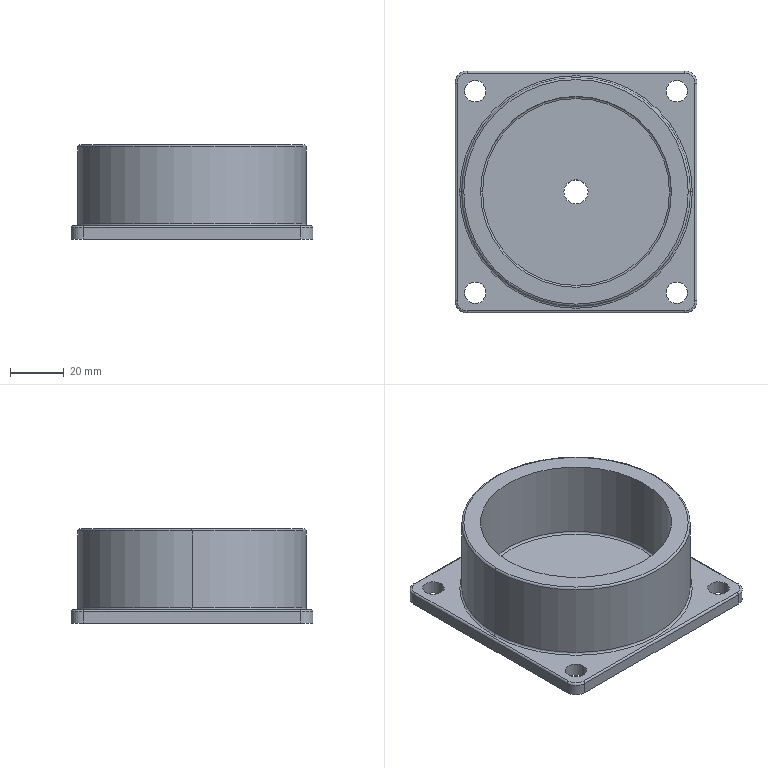Part | SolidWorks | features ICE 4, Extrusion 1, Fillet 1, Scale 1 | 1 solid | 40 faces | box 90 x 90 x 35 mm | volume 90534 mm3 | cylinder 22 | torus 10 | plane 8 | commonest cylinder face diameters 8 x8 9 x6 1.5 x4 71 x2 85 x2
STEP:
#1=CARTESIAN_POINT('',(1.319,-1.476,0.1969));
#2=VERTEX_POINT('',#1);
#3=CARTESIAN_POINT('',(1.634,-1.476,0.1969));
#4=VERTEX_POINT('',#3);
#5=CARTESIAN_POINT('',(1.476,-1.476,0.1969));
#6=DIRECTION('',(0.,0.,1.));
#7=DIRECTION('',(1.,0.,0.));
#8=AXIS2_PLACEMENT_3D('',#5,#6,#7);
#9=CIRCLE('',#8,0.1575);
#10=EDGE_CURVE('',#2,#4,#9,.T.);
#11=ORIENTED_EDGE('',*,*,#10,.T.);
#12=CARTESIAN_POINT('',(1.634,-1.476,0.));
#13=VERTEX_POINT('',#12);
#14=CARTESIAN_POINT('',(1.634,-1.476,0.3937));
#15=DIRECTION('',(0.,0.,-1.));
#16=VECTOR('',#15,39.37);
#17=LINE('',#14,#16);
#18=EDGE_CURVE('',#4,#13,#17,.T.);
#19=ORIENTED_EDGE('',*,*,#18,.T.);
#20=CARTESIAN_POINT('',(1.319,-1.476,0.));
#21=VERTEX_POINT('',#20);
#22=CARTESIAN_POINT('',(1.476,-1.476,0.));
#23=DIRECTION('',(0.,0.,-1.));
#24=DIRECTION('',(1.,0.,0.));
#25=AXIS2_PLACEMENT_3D('',#22,#23,#24);
#26=CIRCLE('',#25,0.1575);
#27=EDGE_CURVE('',#13,#21,#26,.T.);
#28=ORIENTED_EDGE('',*,*,#27,.T.);
#29=CARTESIAN_POINT('',(1.319,-1.476,0.3937));
#30=DIRECTION('',(0.,0.,-1.));
#31=VECTOR('',#30,39.37);
#32=LINE('',#29,#31);
#33=EDGE_CURVE('',#2,#21,#32,.T.);
#34=ORIENTED_EDGE('',*,*,#33,.F.);
#35=EDGE_LOOP('',(#11,#19,#28,#34));
#36=FACE_OUTER_BOUND('',#35,.T.);
#37=CARTESIAN_POINT('',(1.476,-1.476,0.3937));
#38=DIRECTION('',(0.,0.,-1.));
#39=DIRECTION('',(-1.,0.,0.));
#40=AXIS2_PLACEMENT_3D('',#37,#38,#39);
#41=CYLINDRICAL_SURFACE('',#40,0.1575);
#42=ADVANCED_FACE('',(#36),#41,.F.);
#43=CARTESIAN_POINT('',(-1.634,1.476,0.1969));
#44=VERTEX_POINT('',#43);
#45=CARTESIAN_POINT('',(-1.319,1.476,0.1969));
#46=VERTEX_POINT('',#45);
#47=CARTESIAN_POINT('',(-1.476,1.476,0.1969));
#48=DIRECTION('',(0.,0.,1.));
#49=DIRECTION('',(1.,0.,0.));
#50=AXIS2_PLACEMENT_3D('',#47,#48,#49);
#51=CIRCLE('',#50,0.1575);
#52=EDGE_CURVE('',#44,#46,#51,.T.);
#53=ORIENTED_EDGE('',*,*,#52,.T.);
#54=CARTESIAN_POINT('',(-1.319,1.476,0.));
#55=VERTEX_POINT('',#54);
#56=CARTESIAN_POINT('',(-1.319,1.476,0.3937));
#57=DIRECTION('',(0.,0.,-1.));
#58=VECTOR('',#57,39.37);
#59=LINE('',#56,#58);
#60=EDGE_CURVE('',#46,#55,#59,.T.);
#61=ORIENTED_EDGE('',*,*,#60,.T.);
#62=CARTESIAN_POINT('',(-1.634,1.476,0.));
#63=VERTEX_POINT('',#62);
#64=CARTESIAN_POINT('',(-1.476,1.476,0.));
#65=DIRECTION('',(0.,0.,-1.));
#66=DIRECTION('',(1.,0.,0.));
#67=AXIS2_PLACEMENT_3D('',#64,#65,#66);
#68=CIRCLE('',#67,0.1575);
#69=EDGE_CURVE('',#55,#63,#68,.T.);
#70=ORIENTED_EDGE('',*,*,#69,.T.);
#71=CARTESIAN_POINT('',(-1.634,1.476,0.3937));
#72=DIRECTION('',(0.,0.,-1.));
#73=VECTOR('',#72,39.37);
#74=LINE('',#71,#73);
#75=EDGE_CURVE('',#44,#63,#74,.T.);
#76=ORIENTED_EDGE('',*,*,#75,.F.);
#77=EDGE_LOOP('',(#53,#61,#70,#76));
#78=FACE_OUTER_BOUND('',#77,.T.);
#79=CARTESIAN_POINT('',(-1.476,1.476,0.3937));
#80=DIRECTION('',(0.,0.,-1.));
#81=DIRECTION('',(-1.,0.,0.));
#82=AXIS2_PLACEMENT_3D('',#79,#80,#81);
#83=CYLINDRICAL_SURFACE('',#82,0.1575);
#84=ADVANCED_FACE('',(#78),#83,.F.);
#85=CARTESIAN_POINT('',(-1.634,-1.476,0.1969));
#86=VERTEX_POINT('',#85);
#87=CARTESIAN_POINT('',(-1.319,-1.476,0.1969));
#88=VERTEX_POINT('',#87);
#89=CARTESIAN_POINT('',(-1.476,-1.476,0.1969));
#90=DIRECTION('',(0.,0.,1.));
#91=DIRECTION('',(1.,0.,0.));
#92=AXIS2_PLACEMENT_3D('',#89,#90,#91);
#93=CIRCLE('',#92,0.1575);
#94=EDGE_CURVE('',#86,#88,#93,.T.);
#95=ORIENTED_EDGE('',*,*,#94,.T.);
#96=CARTESIAN_POINT('',(-1.319,-1.476,0.));
#97=VERTEX_POINT('',#96);
#98=CARTESIAN_POINT('',(-1.319,-1.476,0.3937));
#99=DIRECTION('',(0.,0.,-1.));
#100=VECTOR('',#99,39.37);
#101=LINE('',#98,#100);
#102=EDGE_CURVE('',#88,#97,#101,.T.);
#103=ORIENTED_EDGE('',*,*,#102,.T.);
#104=CARTESIAN_POINT('',(-1.634,-1.476,0.));
#105=VERTEX_POINT('',#104);
#106=CARTESIAN_POINT('',(-1.476,-1.476,0.));
#107=DIRECTION('',(0.,0.,-1.));
#108=DIRECTION('',(-1.,0.,0.));
#109=AXIS2_PLACEMENT_3D('',#106,#107,#108);
#110=CIRCLE('',#109,0.1575);
#111=EDGE_CURVE('',#97,#105,#110,.T.);
#112=ORIENTED_EDGE('',*,*,#111,.T.);
#113=CARTESIAN_POINT('',(-1.634,-1.476,0.3937));
#114=DIRECTION('',(0.,0.,-1.));
#115=VECTOR('',#114,39.37);
#116=LINE('',#113,#115);
#117=EDGE_CURVE('',#86,#105,#116,.T.);
#118=ORIENTED_EDGE('',*,*,#117,.F.);
#119=EDGE_LOOP('',(#95,#103,#112,#118));
#120=FACE_OUTER_BOUND('',#119,.T.);
#121=CARTESIAN_POINT('',(-1.476,-1.476,0.3937));
#122=DIRECTION('',(0.,0.,-1.));
#123=DIRECTION('',(-1.,0.,0.));
#124=AXIS2_PLACEMENT_3D('',#121,#122,#123);
#125=CYLINDRICAL_SURFACE('',#124,0.1575);
#126=ADVANCED_FACE('',(#120),#125,.F.);
#127=CARTESIAN_POINT('',(1.319,1.476,0.1969));
#128=VERTEX_POINT('',#127);
#129=CARTESIAN_POINT('',(1.634,1.476,0.1969));
#130=VERTEX_POINT('',#129);
#131=CARTESIAN_POINT('',(1.476,1.476,0.1969));
#132=DIRECTION('',(0.,0.,1.));
#133=DIRECTION('',(1.,0.,0.));
#134=AXIS2_PLACEMENT_3D('',#131,#132,#133);
#135=CIRCLE('',#134,0.1575);
#136=EDGE_CURVE('',#128,#130,#135,.T.);
#137=ORIENTED_EDGE('',*,*,#136,.T.);
#138=CARTESIAN_POINT('',(1.634,1.476,0.));
#139=VERTEX_POINT('',#138);
#140=CARTESIAN_POINT('',(1.634,1.476,0.3937));
#141=DIRECTION('',(0.,0.,-1.));
#142=VECTOR('',#141,39.37);
#143=LINE('',#140,#142);
#144=EDGE_CURVE('',#130,#139,#143,.T.);
#145=ORIENTED_EDGE('',*,*,#144,.T.);
#146=CARTESIAN_POINT('',(1.319,1.476,0.));
#147=VERTEX_POINT('',#146);
#148=CARTESIAN_POINT('',(1.476,1.476,0.));
#149=DIRECTION('',(0.,0.,-1.));
#150=DIRECTION('',(-1.,0.,0.));
#151=AXIS2_PLACEMENT_3D('',#148,#149,#150);
#152=CIRCLE('',#151,0.1575);
#153=EDGE_CURVE('',#139,#147,#152,.T.);
#154=ORIENTED_EDGE('',*,*,#153,.T.);
#155=CARTESIAN_POINT('',(1.319,1.476,0.3937));
#156=DIRECTION('',(0.,0.,-1.));
#157=VECTOR('',#156,39.37);
#158=LINE('',#155,#157);
#159=EDGE_CURVE('',#128,#147,#158,.T.);
#160=ORIENTED_EDGE('',*,*,#159,.F.);
#161=EDGE_LOOP('',(#137,#145,#154,#160));
#162=FACE_OUTER_BOUND('',#161,.T.);
#163=CARTESIAN_POINT('',(1.476,1.476,0.3937));
#164=DIRECTION('',(0.,0.,-1.));
#165=DIRECTION('',(-1.,0.,0.));
#166=AXIS2_PLACEMENT_3D('',#163,#164,#165);
#167=CYLINDRICAL_SURFACE('',#166,0.1575);
#168=ADVANCED_FACE('',(#162),#167,.F.);
#169=CARTESIAN_POINT('',(-1.673,0.,0.2264));
#170=VERTEX_POINT('',#169);
#171=CARTESIAN_POINT('',(1.673,0.,0.2264));
#172=VERTEX_POINT('',#171);
#173=CARTESIAN_POINT('',(0.,0.,0.2264));
#174=DIRECTION('',(0.,0.,1.));
#175=DIRECTION('',(1.,0.,0.));
#176=AXIS2_PLACEMENT_3D('',#173,#174,#175);
#177=CIRCLE('',#176,1.673);
#178=EDGE_CURVE('',#170,#172,#177,.T.);
#179=ORIENTED_EDGE('',*,*,#178,.F.);
#180=CARTESIAN_POINT('',(-1.703,0.,0.1969));
#181=VERTEX_POINT('',#180);
#182=CARTESIAN_POINT('',(-1.703,0.,0.2264));
#183=DIRECTION('',(0.,1.,0.));
#184=DIRECTION('',(-1.,0.,0.));
#185=AXIS2_PLACEMENT_3D('',#182,#183,#184);
#186=CIRCLE('',#185,0.02953);
#187=EDGE_CURVE('',#170,#181,#186,.T.);
#188=ORIENTED_EDGE('',*,*,#187,.T.);
#189=CARTESIAN_POINT('',(1.703,0.,0.1969));
#190=VERTEX_POINT('',#189);
#191=CARTESIAN_POINT('',(0.,0.,0.1969));
#192=DIRECTION('',(0.,0.,-1.));
#193=DIRECTION('',(1.,0.,0.));
#194=AXIS2_PLACEMENT_3D('',#191,#192,#193);
#195=CIRCLE('',#194,1.703);
#196=EDGE_CURVE('',#190,#181,#195,.T.);
#197=ORIENTED_EDGE('',*,*,#196,.F.);
#198=CARTESIAN_POINT('',(1.703,0.,0.2264));
#199=DIRECTION('',(0.,-1.,0.));
#200=DIRECTION('',(0.,0.,-1.));
#201=AXIS2_PLACEMENT_3D('',#198,#199,#200);
#202=CIRCLE('',#201,0.02953);
#203=EDGE_CURVE('',#172,#190,#202,.T.);
#204=ORIENTED_EDGE('',*,*,#203,.F.);
#205=EDGE_LOOP('',(#179,#188,#197,#204));
#206=FACE_OUTER_BOUND('',#205,.T.);
#207=CARTESIAN_POINT('',(0.,0.,0.2264));
#208=DIRECTION('',(0.,0.,1.));
#209=DIRECTION('',(1.,0.,0.));
#210=AXIS2_PLACEMENT_3D('',#207,#208,#209);
#211=TOROIDAL_SURFACE('',#210,1.703,0.02953);
#212=ADVANCED_FACE('',(#206),#211,.F.);
#213=CARTESIAN_POINT('',(-1.368,0.,0.1969));
#214=VERTEX_POINT('',#213);
#215=CARTESIAN_POINT('',(1.368,0.,0.1969));
#216=VERTEX_POINT('',#215);
#217=CARTESIAN_POINT('',(0.,0.,0.1969));
#218=DIRECTION('',(0.,0.,1.));
#219=DIRECTION('',(1.,0.,0.));
#220=AXIS2_PLACEMENT_3D('',#217,#218,#219);
#221=CIRCLE('',#220,1.368);
#222=EDGE_CURVE('',#214,#216,#221,.T.);
#223=ORIENTED_EDGE('',*,*,#222,.F.);
#224=CARTESIAN_POINT('',(-1.398,0.,0.2264));
#225=VERTEX_POINT('',#224);
#226=CARTESIAN_POINT('',(-1.368,0.,0.2264));
#227=DIRECTION('',(0.,1.,0.));
#228=DIRECTION('',(-1.,0.,0.));
#229=AXIS2_PLACEMENT_3D('',#226,#227,#228);
#230=CIRCLE('',#229,0.02953);
#231=EDGE_CURVE('',#214,#225,#230,.T.);
#232=ORIENTED_EDGE('',*,*,#231,.T.);
#233=CARTESIAN_POINT('',(1.398,0.,0.2264));
#234=VERTEX_POINT('',#233);
#235=CARTESIAN_POINT('',(0.,0.,0.2264));
#236=DIRECTION('',(0.,0.,-1.));
#237=DIRECTION('',(1.,0.,0.));
#238=AXIS2_PLACEMENT_3D('',#235,#236,#237);
#239=CIRCLE('',#238,1.398);
#240=EDGE_CURVE('',#234,#225,#239,.T.);
#241=ORIENTED_EDGE('',*,*,#240,.F.);
#242=CARTESIAN_POINT('',(1.368,0.,0.2264));
#243=DIRECTION('',(0.,-1.,0.));
#244=DIRECTION('',(0.,0.,-1.));
#245=AXIS2_PLACEMENT_3D('',#242,#243,#244);
#246=CIRCLE('',#245,0.02953);
#247=EDGE_CURVE('',#216,#234,#246,.T.);
#248=ORIENTED_EDGE('',*,*,#247,.F.);
#249=EDGE_LOOP('',(#223,#232,#241,#248));
#250=FACE_OUTER_BOUND('',#249,.T.);
#251=CARTESIAN_POINT('',(0.,0.,0.2264));
#252=DIRECTION('',(0.,0.,1.));
#253=DIRECTION('',(1.,0.,0.));
#254=AXIS2_PLACEMENT_3D('',#251,#252,#253);
#255=TOROIDAL_SURFACE('',#254,1.368,0.02953);
#256=ADVANCED_FACE('',(#250),#255,.F.);
#257=CARTESIAN_POINT('',(-1.673,0.,1.348));
#258=VERTEX_POINT('',#257);
#259=CARTESIAN_POINT('',(1.673,0.,1.348));
#260=VERTEX_POINT('',#259);
#261=CARTESIAN_POINT('',(0.,0.,1.348));
#262=DIRECTION('',(0.,0.,-1.));
#263=DIRECTION('',(1.,0.,0.));
#264=AXIS2_PLACEMENT_3D('',#261,#262,#263);
#265=CIRCLE('',#264,1.673);
#266=EDGE_CURVE('',#258,#260,#265,.T.);
#267=ORIENTED_EDGE('',*,*,#266,.F.);
#268=CARTESIAN_POINT('',(-1.644,0.,1.378));
#269=VERTEX_POINT('',#268);
#270=CARTESIAN_POINT('',(-1.644,0.,1.348));
#271=DIRECTION('',(0.,1.,0.));
#272=DIRECTION('',(-1.,0.,0.));
#273=AXIS2_PLACEMENT_3D('',#270,#271,#272);
#274=CIRCLE('',#273,0.02953);
#275=EDGE_CURVE('',#258,#269,#274,.T.);
#276=ORIENTED_EDGE('',*,*,#275,.T.);
#277=CARTESIAN_POINT('',(1.644,0.,1.378));
#278=VERTEX_POINT('',#277);
#279=CARTESIAN_POINT('',(0.,0.,1.378));
#280=DIRECTION('',(0.,0.,1.));
#281=DIRECTION('',(1.,0.,0.));
#282=AXIS2_PLACEMENT_3D('',#279,#280,#281);
#283=CIRCLE('',#282,1.644);
#284=EDGE_CURVE('',#278,#269,#283,.T.);
#285=ORIENTED_EDGE('',*,*,#284,.F.);
#286=CARTESIAN_POINT('',(1.644,0.,1.348));
#287=DIRECTION('',(0.,-1.,0.));
#288=DIRECTION('',(0.,0.,-1.));
#289=AXIS2_PLACEMENT_3D('',#286,#287,#288);
#290=CIRCLE('',#289,0.02953);
#291=EDGE_CURVE('',#260,#278,#290,.T.);
#292=ORIENTED_EDGE('',*,*,#291,.F.);
#293=EDGE_LOOP('',(#267,#276,#285,#292));
#294=FACE_OUTER_BOUND('',#293,.T.);
#295=CARTESIAN_POINT('',(0.,0.,1.348));
#296=DIRECTION('',(0.,0.,1.));
#297=DIRECTION('',(1.,0.,0.));
#298=AXIS2_PLACEMENT_3D('',#295,#296,#297);
#299=TOROIDAL_SURFACE('',#298,1.644,0.02953);
#300=ADVANCED_FACE('',(#294),#299,.T.);
#301=ORIENTED_EDGE('',*,*,#240,.T.);
#302=CARTESIAN_POINT('',(-1.398,0.,1.378));
#303=VERTEX_POINT('',#302);
#304=CARTESIAN_POINT('',(-1.398,0.,0.1969));
#305=DIRECTION('',(0.,0.,1.));
#306=VECTOR('',#305,39.37);
#307=LINE('',#304,#306);
#308=EDGE_CURVE('',#225,#303,#307,.T.);
#309=ORIENTED_EDGE('',*,*,#308,.T.);
#310=CARTESIAN_POINT('',(1.398,0.,1.378));
#311=VERTEX_POINT('',#310);
#312=CARTESIAN_POINT('',(0.,0.,1.378));
#313=DIRECTION('',(0.,0.,1.));
#314=DIRECTION('',(1.,0.,0.));
#315=AXIS2_PLACEMENT_3D('',#312,#313,#314);
#316=CIRCLE('',#315,1.398);
#317=EDGE_CURVE('',#303,#311,#316,.T.);
#318=ORIENTED_EDGE('',*,*,#317,.T.);
#319=CARTESIAN_POINT('',(1.398,0.,0.1969));
#320=DIRECTION('',(0.,0.,1.));
#321=VECTOR('',#320,39.37);
#322=LINE('',#319,#321);
#323=EDGE_CURVE('',#234,#311,#322,.T.);
#324=ORIENTED_EDGE('',*,*,#323,.F.);
#325=EDGE_LOOP('',(#301,#309,#318,#324));
#326=FACE_OUTER_BOUND('',#325,.T.);
#327=CARTESIAN_POINT('',(0.,0.,0.1969));
#328=DIRECTION('',(0.,0.,1.));
#329=DIRECTION('',(1.,0.,0.));
#330=AXIS2_PLACEMENT_3D('',#327,#328,#329);
#331=CYLINDRICAL_SURFACE('',#330,1.398);
#332=ADVANCED_FACE('',(#326),#331,.F.);
#333=ORIENTED_EDGE('',*,*,#266,.T.);
#334=CARTESIAN_POINT('',(1.673,0.,1.378));
#335=DIRECTION('',(0.,0.,-1.));
#336=VECTOR('',#335,39.37);
#337=LINE('',#334,#336);
#338=EDGE_CURVE('',#260,#172,#337,.T.);
#339=ORIENTED_EDGE('',*,*,#338,.T.);
#340=CARTESIAN_POINT('',(0.,0.,0.2264));
#341=DIRECTION('',(0.,0.,1.));
#342=DIRECTION('',(1.,0.,0.));
#343=AXIS2_PLACEMENT_3D('',#340,#341,#342);
#344=CIRCLE('',#343,1.673);
#345=EDGE_CURVE('',#172,#170,#344,.T.);
#346=ORIENTED_EDGE('',*,*,#345,.T.);
#347=CARTESIAN_POINT('',(-1.673,0.,1.378));
#348=DIRECTION('',(0.,0.,-1.));
#349=VECTOR('',#348,39.37);
#350=LINE('',#347,#349);
#351=EDGE_CURVE('',#258,#170,#350,.T.);
#352=ORIENTED_EDGE('',*,*,#351,.F.);
#353=EDGE_LOOP('',(#333,#339,#346,#352));
#354=FACE_OUTER_BOUND('',#353,.T.);
#355=CARTESIAN_POINT('',(0.,0.,1.378));
#356=DIRECTION('',(0.,0.,-1.));
#357=DIRECTION('',(-1.,0.,0.));
#358=AXIS2_PLACEMENT_3D('',#355,#356,#357);
#359=CYLINDRICAL_SURFACE('',#358,1.673);
#360=ADVANCED_FACE('',(#354),#359,.T.);
#361=CARTESIAN_POINT('',(-0.1772,0.,0.1969));
#362=VERTEX_POINT('',#361);
#363=CARTESIAN_POINT('',(0.1772,0.,0.1969));
#364=VERTEX_POINT('',#363);
#365=CARTESIAN_POINT('',(0.,0.,0.1969));
#366=DIRECTION('',(0.,0.,1.));
#367=DIRECTION('',(1.,0.,0.));
#368=AXIS2_PLACEMENT_3D('',#365,#366,#367);
#369=CIRCLE('',#368,0.1772);
#370=EDGE_CURVE('',#362,#364,#369,.T.);
#371=ORIENTED_EDGE('',*,*,#370,.T.);
#372=CARTESIAN_POINT('',(0.1772,0.,0.));
#373=VERTEX_POINT('',#372);
#374=CARTESIAN_POINT('',(0.1772,0.,0.1969));
#375=DIRECTION('',(0.,0.,-1.));
#376=VECTOR('',#375,39.37);
#377=LINE('',#374,#376);
#378=EDGE_CURVE('',#364,#373,#377,.T.);
#379=ORIENTED_EDGE('',*,*,#378,.T.);
#380=CARTESIAN_POINT('',(-0.1772,0.,0.));
#381=VERTEX_POINT('',#380);
#382=CARTESIAN_POINT('',(0.,0.,0.));
#383=DIRECTION('',(0.,0.,1.));
#384=DIRECTION('',(1.,0.,0.));
#385=AXIS2_PLACEMENT_3D('',#382,#383,#384);
#386=CIRCLE('',#385,0.1772);
#387=EDGE_CURVE('',#381,#373,#386,.T.);
#388=ORIENTED_EDGE('',*,*,#387,.F.);
#389=CARTESIAN_POINT('',(-0.1772,0.,0.1969));
#390=DIRECTION('',(0.,0.,-1.));
#391=VECTOR('',#390,39.37);
#392=LINE('',#389,#391);
#393=EDGE_CURVE('',#362,#381,#392,.T.);
#394=ORIENTED_EDGE('',*,*,#393,.F.);
#395=EDGE_LOOP('',(#371,#379,#388,#394));
#396=FACE_OUTER_BOUND('',#395,.T.);
#397=CARTESIAN_POINT('',(0.,0.,0.1969));
#398=DIRECTION('',(0.,0.,-1.));
#399=DIRECTION('',(-1.,0.,0.));
#400=AXIS2_PLACEMENT_3D('',#397,#398,#399);
#401=CYLINDRICAL_SURFACE('',#400,0.1772);
#402=ADVANCED_FACE('',(#396),#401,.F.);
#403=ORIENTED_EDGE('',*,*,#10,.F.);
#404=CARTESIAN_POINT('',(1.476,-1.476,0.1969));
#405=DIRECTION('',(0.,0.,1.));
#406=DIRECTION('',(1.,0.,0.));
#407=AXIS2_PLACEMENT_3D('',#404,#405,#406);
#408=CIRCLE('',#407,0.1575);
#409=EDGE_CURVE('',#4,#2,#408,.T.);
#410=ORIENTED_EDGE('',*,*,#409,.F.);
#411=EDGE_LOOP('',(#403,#410));
#412=FACE_BOUND('',#411,.T.);
#413=ORIENTED_EDGE('',*,*,#52,.F.);
#414=CARTESIAN_POINT('',(-1.476,1.476,0.1969));
#415=DIRECTION('',(0.,0.,1.));
#416=DIRECTION('',(1.,0.,0.));
#417=AXIS2_PLACEMENT_3D('',#414,#415,#416);
#418=CIRCLE('',#417,0.1575);
#419=EDGE_CURVE('',#46,#44,#418,.T.);
#420=ORIENTED_EDGE('',*,*,#419,.F.);
#421=EDGE_LOOP('',(#413,#420));
#422=FACE_BOUND('',#421,.T.);
#423=ORIENTED_EDGE('',*,*,#94,.F.);
#424=CARTESIAN_POINT('',(-1.476,-1.476,0.1969));
#425=DIRECTION('',(0.,0.,1.));
#426=DIRECTION('',(1.,0.,0.));
#427=AXIS2_PLACEMENT_3D('',#424,#425,#426);
#428=CIRCLE('',#427,0.1575);
#429=EDGE_CURVE('',#88,#86,#428,.T.);
#430=ORIENTED_EDGE('',*,*,#429,.F.);
#431=EDGE_LOOP('',(#423,#430));
#432=FACE_BOUND('',#431,.T.);
#433=ORIENTED_EDGE('',*,*,#136,.F.);
#434=CARTESIAN_POINT('',(1.476,1.476,0.1969));
#435=DIRECTION('',(0.,0.,1.));
#436=DIRECTION('',(1.,0.,0.));
#437=AXIS2_PLACEMENT_3D('',#434,#435,#436);
#438=CIRCLE('',#437,0.1575);
#439=EDGE_CURVE('',#130,#128,#438,.T.);
#440=ORIENTED_EDGE('',*,*,#439,.F.);
#441=EDGE_LOOP('',(#433,#440));
#442=FACE_BOUND('',#441,.T.);
#443=CARTESIAN_POINT('',(-1.594,-1.742,0.1969));
#444=VERTEX_POINT('',#443);
#445=CARTESIAN_POINT('',(1.594,-1.742,0.1969));
#446=VERTEX_POINT('',#445);
#447=CARTESIAN_POINT('',(1.594,-1.742,0.1969));
#448=DIRECTION('',(1.,0.,0.));
#449=VECTOR('',#448,39.37);
#450=LINE('',#447,#449);
#451=EDGE_CURVE('',#444,#446,#450,.T.);
#452=ORIENTED_EDGE('',*,*,#451,.T.);
#453=CARTESIAN_POINT('',(1.742,-1.594,0.1969));
#454=VERTEX_POINT('',#453);
#455=CARTESIAN_POINT('',(1.594,-1.594,0.1969));
#456=DIRECTION('',(0.,0.,1.));
#457=DIRECTION('',(1.,0.,0.));
#458=AXIS2_PLACEMENT_3D('',#455,#456,#457);
#459=CIRCLE('',#458,0.1476);
#460=EDGE_CURVE('',#446,#454,#459,.T.);
#461=ORIENTED_EDGE('',*,*,#460,.T.);
#462=CARTESIAN_POINT('',(1.742,1.594,0.1969));
#463=VERTEX_POINT('',#462);
#464=CARTESIAN_POINT('',(1.742,1.594,0.1969));
#465=DIRECTION('',(0.,1.,0.));
#466=VECTOR('',#465,39.37);
#467=LINE('',#464,#466);
#468=EDGE_CURVE('',#454,#463,#467,.T.);
#469=ORIENTED_EDGE('',*,*,#468,.T.);
#470=CARTESIAN_POINT('',(1.594,1.742,0.1969));
#471=VERTEX_POINT('',#470);
#472=CARTESIAN_POINT('',(1.594,1.594,0.1969));
#473=DIRECTION('',(0.,0.,1.));
#474=DIRECTION('',(1.,0.,0.));
#475=AXIS2_PLACEMENT_3D('',#472,#473,#474);
#476=CIRCLE('',#475,0.1476);
#477=EDGE_CURVE('',#463,#471,#476,.T.);
#478=ORIENTED_EDGE('',*,*,#477,.T.);
#479=CARTESIAN_POINT('',(-1.594,1.742,0.1969));
#480=VERTEX_POINT('',#479);
#481=CARTESIAN_POINT('',(-1.594,1.742,0.1969));
#482=DIRECTION('',(-1.,0.,0.));
#483=VECTOR('',#482,39.37);
#484=LINE('',#481,#483);
#485=EDGE_CURVE('',#471,#480,#484,.T.);
#486=ORIENTED_EDGE('',*,*,#485,.T.);
#487=CARTESIAN_POINT('',(-1.742,1.594,0.1969));
#488=VERTEX_POINT('',#487);
#489=CARTESIAN_POINT('',(-1.594,1.594,0.1969));
#490=DIRECTION('',(0.,0.,1.));
#491=DIRECTION('',(1.,0.,0.));
#492=AXIS2_PLACEMENT_3D('',#489,#490,#491);
#493=CIRCLE('',#492,0.1476);
#494=EDGE_CURVE('',#480,#488,#493,.T.);
#495=ORIENTED_EDGE('',*,*,#494,.T.);
#496=CARTESIAN_POINT('',(-1.742,-1.594,0.1969));
#497=VERTEX_POINT('',#496);
#498=CARTESIAN_POINT('',(-1.742,-1.594,0.1969));
#499=DIRECTION('',(0.,-1.,0.));
#500=VECTOR('',#499,39.37);
#501=LINE('',#498,#500);
#502=EDGE_CURVE('',#488,#497,#501,.T.);
#503=ORIENTED_EDGE('',*,*,#502,.T.);
#504=CARTESIAN_POINT('',(-1.594,-1.594,0.1969));
#505=DIRECTION('',(0.,0.,1.));
#506=DIRECTION('',(1.,0.,0.));
#507=AXIS2_PLACEMENT_3D('',#504,#505,#506);
#508=CIRCLE('',#507,0.1476);
#509=EDGE_CURVE('',#497,#444,#508,.T.);
#510=ORIENTED_EDGE('',*,*,#509,.T.);
#511=EDGE_LOOP('',(#452,#461,#469,#478,#486,#495,#503,#510));
#512=FACE_OUTER_BOUND('',#511,.T.);
#513=ORIENTED_EDGE('',*,*,#196,.T.);
#514=CARTESIAN_POINT('',(0.,0.,0.1969));
#515=DIRECTION('',(0.,0.,-1.));
#516=DIRECTION('',(1.,0.,0.));
#517=AXIS2_PLACEMENT_3D('',#514,#515,#516);
#518=CIRCLE('',#517,1.703);
#519=EDGE_CURVE('',#181,#190,#518,.T.);
#520=ORIENTED_EDGE('',*,*,#519,.T.);
#521=EDGE_LOOP('',(#513,#520));
#522=FACE_BOUND('',#521,.T.);
#523=CARTESIAN_POINT('',(1.594,-1.594,0.1969));
#524=DIRECTION('',(0.,0.,1.));
#525=DIRECTION('',(1.,0.,0.));
#526=AXIS2_PLACEMENT_3D('',#523,#524,#525);
#527=PLANE('',#526);
#528=ADVANCED_FACE('',(#412,#422,#432,#442,#512,#522),#527,.T.);
#529=CARTESIAN_POINT('',(1.476,-1.476,0.));
#530=DIRECTION('',(0.,0.,-1.));
#531=DIRECTION('',(1.,0.,0.));
#532=AXIS2_PLACEMENT_3D('',#529,#530,#531);
#533=CIRCLE('',#532,0.1575);
#534=EDGE_CURVE('',#21,#13,#533,.T.);
#535=ORIENTED_EDGE('',*,*,#534,.F.);
#536=ORIENTED_EDGE('',*,*,#27,.F.);
#537=EDGE_LOOP('',(#535,#536));
#538=FACE_BOUND('',#537,.T.);
#539=CARTESIAN_POINT('',(-1.476,1.476,0.));
#540=DIRECTION('',(0.,0.,-1.));
#541=DIRECTION('',(1.,0.,0.));
#542=AXIS2_PLACEMENT_3D('',#539,#540,#541);
#543=CIRCLE('',#542,0.1575);
#544=EDGE_CURVE('',#63,#55,#543,.T.);
#545=ORIENTED_EDGE('',*,*,#544,.F.);
#546=ORIENTED_EDGE('',*,*,#69,.F.);
#547=EDGE_LOOP('',(#545,#546));
#548=FACE_BOUND('',#547,.T.);
#549=CARTESIAN_POINT('',(-1.476,-1.476,0.));
#550=DIRECTION('',(0.,0.,-1.));
#551=DIRECTION('',(-1.,0.,0.));
#552=AXIS2_PLACEMENT_3D('',#549,#550,#551);
#553=CIRCLE('',#552,0.1575);
#554=EDGE_CURVE('',#105,#97,#553,.T.);
#555=ORIENTED_EDGE('',*,*,#554,.F.);
#556=ORIENTED_EDGE('',*,*,#111,.F.);
#557=EDGE_LOOP('',(#555,#556));
#558=FACE_BOUND('',#557,.T.);
#559=CARTESIAN_POINT('',(1.476,1.476,0.));
#560=DIRECTION('',(0.,0.,-1.));
#561=DIRECTION('',(-1.,0.,0.));
#562=AXIS2_PLACEMENT_3D('',#559,#560,#561);
#563=CIRCLE('',#562,0.1575);
#564=EDGE_CURVE('',#147,#139,#563,.T.);
#565=ORIENTED_EDGE('',*,*,#564,.F.);
#566=ORIENTED_EDGE('',*,*,#153,.F.);
#567=EDGE_LOOP('',(#565,#566));
#568=FACE_BOUND('',#567,.T.);
#569=CARTESIAN_POINT('',(1.594,-1.772,0.));
#570=VERTEX_POINT('',#569);
#571=CARTESIAN_POINT('',(1.772,-1.594,0.));
#572=VERTEX_POINT('',#571);
#573=CARTESIAN_POINT('',(1.594,-1.594,0.));
#574=DIRECTION('',(0.,0.,1.));
#575=DIRECTION('',(1.,0.,0.));
#576=AXIS2_PLACEMENT_3D('',#573,#574,#575);
#577=CIRCLE('',#576,0.1772);
#578=EDGE_CURVE('',#570,#572,#577,.T.);
#579=ORIENTED_EDGE('',*,*,#578,.F.);
#580=CARTESIAN_POINT('',(-1.594,-1.772,0.));
#581=VERTEX_POINT('',#580);
#582=CARTESIAN_POINT('',(-1.594,-1.772,0.));
#583=DIRECTION('',(1.,0.,0.));
#584=VECTOR('',#583,39.37);
#585=LINE('',#582,#584);
#586=EDGE_CURVE('',#581,#570,#585,.T.);
#587=ORIENTED_EDGE('',*,*,#586,.F.);
#588=CARTESIAN_POINT('',(-1.772,-1.594,0.));
#589=VERTEX_POINT('',#588);
#590=CARTESIAN_POINT('',(-1.594,-1.594,0.));
#591=DIRECTION('',(0.,0.,1.));
#592=DIRECTION('',(-1.,0.,0.));
#593=AXIS2_PLACEMENT_3D('',#590,#591,#592);
#594=CIRCLE('',#593,0.1772);
#595=EDGE_CURVE('',#589,#581,#594,.T.);
#596=ORIENTED_EDGE('',*,*,#595,.F.);
#597=CARTESIAN_POINT('',(-1.772,1.594,0.));
#598=VERTEX_POINT('',#597);
#599=CARTESIAN_POINT('',(-1.772,-1.594,0.));
#600=DIRECTION('',(0.,-1.,0.));
#601=VECTOR('',#600,39.37);
#602=LINE('',#599,#601);
#603=EDGE_CURVE('',#598,#589,#602,.T.);
#604=ORIENTED_EDGE('',*,*,#603,.F.);
#605=CARTESIAN_POINT('',(-1.594,1.772,0.));
#606=VERTEX_POINT('',#605);
#607=CARTESIAN_POINT('',(-1.594,1.594,0.));
#608=DIRECTION('',(0.,0.,1.));
#609=DIRECTION('',(-1.,0.,0.));
#610=AXIS2_PLACEMENT_3D('',#607,#608,#609);
#611=CIRCLE('',#610,0.1772);
#612=EDGE_CURVE('',#606,#598,#611,.T.);
#613=ORIENTED_EDGE('',*,*,#612,.F.);
#614=CARTESIAN_POINT('',(1.594,1.772,0.));
#615=VERTEX_POINT('',#614);
#616=CARTESIAN_POINT('',(-1.594,1.772,0.));
#617=DIRECTION('',(-1.,0.,0.));
#618=VECTOR('',#617,39.37);
#619=LINE('',#616,#618);
#620=EDGE_CURVE('',#615,#606,#619,.T.);
#621=ORIENTED_EDGE('',*,*,#620,.F.);
#622=CARTESIAN_POINT('',(1.772,1.594,0.));
#623=VERTEX_POINT('',#622);
#624=CARTESIAN_POINT('',(1.594,1.594,0.));
#625=DIRECTION('',(0.,0.,1.));
#626=DIRECTION('',(-1.,0.,0.));
#627=AXIS2_PLACEMENT_3D('',#624,#625,#626);
#628=CIRCLE('',#627,0.1772);
#629=EDGE_CURVE('',#623,#615,#628,.T.);
#630=ORIENTED_EDGE('',*,*,#629,.F.);
#631=CARTESIAN_POINT('',(1.772,-1.594,0.));
#632=DIRECTION('',(0.,1.,0.));
#633=VECTOR('',#632,39.37);
#634=LINE('',#631,#633);
#635=EDGE_CURVE('',#572,#623,#634,.T.);
#636=ORIENTED_EDGE('',*,*,#635,.F.);
#637=EDGE_LOOP('',(#579,#587,#596,#604,#613,#621,#630,#636));
#638=FACE_OUTER_BOUND('',#637,.T.);
#639=ORIENTED_EDGE('',*,*,#387,.T.);
#640=CARTESIAN_POINT('',(0.,0.,0.));
#641=DIRECTION('',(0.,0.,1.));
#642=DIRECTION('',(1.,0.,0.));
#643=AXIS2_PLACEMENT_3D('',#640,#641,#642);
#644=CIRCLE('',#643,0.1772);
#645=EDGE_CURVE('',#373,#381,#644,.T.);
#646=ORIENTED_EDGE('',*,*,#645,.T.);
#647=EDGE_LOOP('',(#639,#646));
#648=FACE_BOUND('',#647,.T.);
#649=CARTESIAN_POINT('',(1.594,-1.594,0.));
#650=DIRECTION('',(0.,0.,1.));
#651=DIRECTION('',(1.,0.,0.));
#652=AXIS2_PLACEMENT_3D('',#649,#650,#651);
#653=PLANE('',#652);
#654=ADVANCED_FACE('',(#538,#548,#558,#568,#638,#648),#653,.F.);
#655=CARTESIAN_POINT('',(1.772,-1.594,0.1673));
#656=VERTEX_POINT('',#655);
#657=CARTESIAN_POINT('',(1.772,-1.594,0.1969));
#658=DIRECTION('',(0.,0.,-1.));
#659=VECTOR('',#658,39.37);
#660=LINE('',#657,#659);
#661=EDGE_CURVE('',#656,#572,#660,.T.);
#662=ORIENTED_EDGE('',*,*,#661,.F.);
#663=CARTESIAN_POINT('',(1.594,-1.772,0.1673));
#664=VERTEX_POINT('',#663);
#665=CARTESIAN_POINT('',(1.594,-1.594,0.1673));
#666=DIRECTION('',(0.,0.,-1.));
#667=DIRECTION('',(1.,0.,0.));
#668=AXIS2_PLACEMENT_3D('',#665,#666,#667);
#669=CIRCLE('',#668,0.1772);
#670=EDGE_CURVE('',#656,#664,#669,.T.);
#671=ORIENTED_EDGE('',*,*,#670,.T.);
#672=CARTESIAN_POINT('',(1.594,-1.772,0.1969));
#673=DIRECTION('',(0.,0.,-1.));
#674=VECTOR('',#673,39.37);
#675=LINE('',#672,#674);
#676=EDGE_CURVE('',#664,#570,#675,.T.);
#677=ORIENTED_EDGE('',*,*,#676,.T.);
#678=ORIENTED_EDGE('',*,*,#578,.T.);
#679=EDGE_LOOP('',(#662,#671,#677,#678));
#680=FACE_OUTER_BOUND('',#679,.T.);
#681=CARTESIAN_POINT('',(1.594,-1.594,0.1969));
#682=DIRECTION('',(0.,0.,-1.));
#683=DIRECTION('',(-1.,0.,0.));
#684=AXIS2_PLACEMENT_3D('',#681,#682,#683);
#685=CYLINDRICAL_SURFACE('',#684,0.1772);
#686=ADVANCED_FACE('',(#680),#685,.T.);
#687=CARTESIAN_POINT('',(1.772,1.594,0.1673));
#688=VERTEX_POINT('',#687);
#689=CARTESIAN_POINT('',(1.772,1.594,0.1969));
#690=DIRECTION('',(0.,0.,-1.));
#691=VECTOR('',#690,39.37);
#692=LINE('',#689,#691);
#693=EDGE_CURVE('',#688,#623,#692,.T.);
#694=ORIENTED_EDGE('',*,*,#693,.F.);
#695=CARTESIAN_POINT('',(1.772,-1.594,0.1673));
#696=DIRECTION('',(0.,-1.,0.));
#697=VECTOR('',#696,39.37);
#698=LINE('',#695,#697);
#699=EDGE_CURVE('',#688,#656,#698,.T.);
#700=ORIENTED_EDGE('',*,*,#699,.T.);
#701=ORIENTED_EDGE('',*,*,#661,.T.);
#702=ORIENTED_EDGE('',*,*,#635,.T.);
#703=EDGE_LOOP('',(#694,#700,#701,#702));
#704=FACE_OUTER_BOUND('',#703,.T.);
#705=CARTESIAN_POINT('',(1.772,-1.594,0.1969));
#706=DIRECTION('',(-1.,0.,0.));
#707=DIRECTION('',(0.,0.,1.));
#708=AXIS2_PLACEMENT_3D('',#705,#706,#707);
#709=PLANE('',#708);
#710=ADVANCED_FACE('',(#704),#709,.F.);
#711=CARTESIAN_POINT('',(1.594,1.772,0.1673));
#712=VERTEX_POINT('',#711);
#713=CARTESIAN_POINT('',(1.594,1.772,0.1969));
#714=DIRECTION('',(0.,0.,-1.));
#715=VECTOR('',#714,39.37);
#716=LINE('',#713,#715);
#717=EDGE_CURVE('',#712,#615,#716,.T.);
#718=ORIENTED_EDGE('',*,*,#717,.F.);
#719=CARTESIAN_POINT('',(1.594,1.594,0.1673));
#720=DIRECTION('',(0.,0.,-1.));
#721=DIRECTION('',(1.,0.,0.));
#722=AXIS2_PLACEMENT_3D('',#719,#720,#721);
#723=CIRCLE('',#722,0.1772);
#724=EDGE_CURVE('',#712,#688,#723,.T.);
#725=ORIENTED_EDGE('',*,*,#724,.T.);
#726=ORIENTED_EDGE('',*,*,#693,.T.);
#727=ORIENTED_EDGE('',*,*,#629,.T.);
#728=EDGE_LOOP('',(#718,#725,#726,#727));
#729=FACE_OUTER_BOUND('',#728,.T.);
#730=CARTESIAN_POINT('',(1.594,1.594,0.1969));
#731=DIRECTION('',(0.,0.,-1.));
#732=DIRECTION('',(-1.,0.,0.));
#733=AXIS2_PLACEMENT_3D('',#730,#731,#732);
#734=CYLINDRICAL_SURFACE('',#733,0.1772);
#735=ADVANCED_FACE('',(#729),#734,.T.);
#736=CARTESIAN_POINT('',(-1.594,1.772,0.1673));
#737=VERTEX_POINT('',#736);
#738=CARTESIAN_POINT('',(-1.594,1.772,0.1969));
#739=DIRECTION('',(0.,0.,-1.));
#740=VECTOR('',#739,39.37);
#741=LINE('',#738,#740);
#742=EDGE_CURVE('',#737,#606,#741,.T.);
#743=ORIENTED_EDGE('',*,*,#742,.F.);
#744=CARTESIAN_POINT('',(1.594,1.772,0.1673));
#745=DIRECTION('',(1.,0.,0.));
#746=VECTOR('',#745,39.37);
#747=LINE('',#744,#746);
#748=EDGE_CURVE('',#737,#712,#747,.T.);
#749=ORIENTED_EDGE('',*,*,#748,.T.);
#750=ORIENTED_EDGE('',*,*,#717,.T.);
#751=ORIENTED_EDGE('',*,*,#620,.T.);
#752=EDGE_LOOP('',(#743,#749,#750,#751));
#753=FACE_OUTER_BOUND('',#752,.T.);
#754=CARTESIAN_POINT('',(-1.594,1.772,0.1969));
#755=DIRECTION('',(0.,-1.,0.));
#756=DIRECTION('',(0.,0.,-1.));
#757=AXIS2_PLACEMENT_3D('',#754,#755,#756);
#758=PLANE('',#757);
#759=ADVANCED_FACE('',(#753),#758,.F.);
#760=CARTESIAN_POINT('',(-1.772,1.594,0.1673));
#761=VERTEX_POINT('',#760);
#762=CARTESIAN_POINT('',(-1.772,1.594,0.1969));
#763=DIRECTION('',(0.,0.,-1.));
#764=VECTOR('',#763,39.37);
#765=LINE('',#762,#764);
#766=EDGE_CURVE('',#761,#598,#765,.T.);
#767=ORIENTED_EDGE('',*,*,#766,.F.);
#768=CARTESIAN_POINT('',(-1.594,1.594,0.1673));
#769=DIRECTION('',(0.,0.,-1.));
#770=DIRECTION('',(1.,0.,0.));
#771=AXIS2_PLACEMENT_3D('',#768,#769,#770);
#772=CIRCLE('',#771,0.1772);
#773=EDGE_CURVE('',#761,#737,#772,.T.);
#774=ORIENTED_EDGE('',*,*,#773,.T.);
#775=ORIENTED_EDGE('',*,*,#742,.T.);
#776=ORIENTED_EDGE('',*,*,#612,.T.);
#777=EDGE_LOOP('',(#767,#774,#775,#776));
#778=FACE_OUTER_BOUND('',#777,.T.);
#779=CARTESIAN_POINT('',(-1.594,1.594,0.1969));
#780=DIRECTION('',(0.,0.,-1.));
#781=DIRECTION('',(-1.,0.,0.));
#782=AXIS2_PLACEMENT_3D('',#779,#780,#781);
#783=CYLINDRICAL_SURFACE('',#782,0.1772);
#784=ADVANCED_FACE('',(#778),#783,.T.);
#785=CARTESIAN_POINT('',(-1.772,-1.594,0.1673));
#786=VERTEX_POINT('',#785);
#787=CARTESIAN_POINT('',(-1.772,-1.594,0.1969));
#788=DIRECTION('',(0.,0.,-1.));
#789=VECTOR('',#788,39.37);
#790=LINE('',#787,#789);
#791=EDGE_CURVE('',#786,#589,#790,.T.);
#792=ORIENTED_EDGE('',*,*,#791,.F.);
#793=CARTESIAN_POINT('',(-1.772,1.594,0.1673));
#794=DIRECTION('',(0.,1.,0.));
#795=VECTOR('',#794,39.37);
#796=LINE('',#793,#795);
#797=EDGE_CURVE('',#786,#761,#796,.T.);
#798=ORIENTED_EDGE('',*,*,#797,.T.);
#799=ORIENTED_EDGE('',*,*,#766,.T.);
#800=ORIENTED_EDGE('',*,*,#603,.T.);
#801=EDGE_LOOP('',(#792,#798,#799,#800));
#802=FACE_OUTER_BOUND('',#801,.T.);
#803=CARTESIAN_POINT('',(-1.772,-1.594,0.1969));
#804=DIRECTION('',(1.,0.,0.));
#805=DIRECTION('',(0.,0.,-1.));
#806=AXIS2_PLACEMENT_3D('',#803,#804,#805);
#807=PLANE('',#806);
#808=ADVANCED_FACE('',(#802),#807,.F.);
#809=CARTESIAN_POINT('',(-1.594,-1.772,0.1673));
#810=VERTEX_POINT('',#809);
#811=CARTESIAN_POINT('',(-1.594,-1.772,0.1969));
#812=DIRECTION('',(0.,0.,-1.));
#813=VECTOR('',#812,39.37);
#814=LINE('',#811,#813);
#815=EDGE_CURVE('',#810,#581,#814,.T.);
#816=ORIENTED_EDGE('',*,*,#815,.F.);
#817=CARTESIAN_POINT('',(-1.594,-1.594,0.1673));
#818=DIRECTION('',(0.,0.,-1.));
#819=DIRECTION('',(1.,0.,0.));
#820=AXIS2_PLACEMENT_3D('',#817,#818,#819);
#821=CIRCLE('',#820,0.1772);
#822=EDGE_CURVE('',#810,#786,#821,.T.);
#823=ORIENTED_EDGE('',*,*,#822,.T.);
#824=ORIENTED_EDGE('',*,*,#791,.T.);
#825=ORIENTED_EDGE('',*,*,#595,.T.);
#826=EDGE_LOOP('',(#816,#823,#824,#825));
#827=FACE_OUTER_BOUND('',#826,.T.);
#828=CARTESIAN_POINT('',(-1.594,-1.594,0.1969));
#829=DIRECTION('',(0.,0.,-1.));
#830=DIRECTION('',(-1.,0.,0.));
#831=AXIS2_PLACEMENT_3D('',#828,#829,#830);
#832=CYLINDRICAL_SURFACE('',#831,0.1772);
#833=ADVANCED_FACE('',(#827),#832,.T.);
#834=ORIENTED_EDGE('',*,*,#676,.F.);
#835=CARTESIAN_POINT('',(-1.594,-1.772,0.1673));
#836=DIRECTION('',(-1.,0.,0.));
#837=VECTOR('',#836,39.37);
#838=LINE('',#835,#837);
#839=EDGE_CURVE('',#664,#810,#838,.T.);
#840=ORIENTED_EDGE('',*,*,#839,.T.);
#841=ORIENTED_EDGE('',*,*,#815,.T.);
#842=ORIENTED_EDGE('',*,*,#586,.T.);
#843=EDGE_LOOP('',(#834,#840,#841,#842));
#844=FACE_OUTER_BOUND('',#843,.T.);
#845=CARTESIAN_POINT('',(-1.594,-1.772,0.1969));
#846=DIRECTION('',(0.,1.,0.));
#847=DIRECTION('',(0.,0.,1.));
#848=AXIS2_PLACEMENT_3D('',#845,#846,#847);
#849=PLANE('',#848);
#850=ADVANCED_FACE('',(#844),#849,.F.);
#851=ORIENTED_EDGE('',*,*,#378,.F.);
#852=CARTESIAN_POINT('',(0.,0.,0.1969));
#853=DIRECTION('',(0.,0.,1.));
#854=DIRECTION('',(1.,0.,0.));
#855=AXIS2_PLACEMENT_3D('',#852,#853,#854);
#856=CIRCLE('',#855,0.1772);
#857=EDGE_CURVE('',#364,#362,#856,.T.);
#858=ORIENTED_EDGE('',*,*,#857,.T.);
#859=ORIENTED_EDGE('',*,*,#393,.T.);
#860=ORIENTED_EDGE('',*,*,#645,.F.);
#861=EDGE_LOOP('',(#851,#858,#859,#860));
#862=FACE_OUTER_BOUND('',#861,.T.);
#863=CARTESIAN_POINT('',(0.,0.,0.1969));
#864=DIRECTION('',(0.,0.,-1.));
#865=DIRECTION('',(-1.,0.,0.));
#866=AXIS2_PLACEMENT_3D('',#863,#864,#865);
#867=CYLINDRICAL_SURFACE('',#866,0.1772);
#868=ADVANCED_FACE('',(#862),#867,.F.);
#869=ORIENTED_EDGE('',*,*,#338,.F.);
#870=CARTESIAN_POINT('',(0.,0.,1.348));
#871=DIRECTION('',(0.,0.,-1.));
#872=DIRECTION('',(1.,0.,0.));
#873=AXIS2_PLACEMENT_3D('',#870,#871,#872);
#874=CIRCLE('',#873,1.673);
#875=EDGE_CURVE('',#260,#258,#874,.T.);
#876=ORIENTED_EDGE('',*,*,#875,.T.);
#877=ORIENTED_EDGE('',*,*,#351,.T.);
#878=ORIENTED_EDGE('',*,*,#178,.T.);
#879=EDGE_LOOP('',(#869,#876,#877,#878));
#880=FACE_OUTER_BOUND('',#879,.T.);
#881=CARTESIAN_POINT('',(0.,0.,1.378));
#882=DIRECTION('',(0.,0.,-1.));
#883=DIRECTION('',(-1.,0.,0.));
#884=AXIS2_PLACEMENT_3D('',#881,#882,#883);
#885=CYLINDRICAL_SURFACE('',#884,1.673);
#886=ADVANCED_FACE('',(#880),#885,.T.);
#887=ORIENTED_EDGE('',*,*,#284,.T.);
#888=CARTESIAN_POINT('',(0.,0.,1.378));
#889=DIRECTION('',(0.,0.,1.));
#890=DIRECTION('',(1.,0.,0.));
#891=AXIS2_PLACEMENT_3D('',#888,#889,#890);
#892=CIRCLE('',#891,1.644);
#893=EDGE_CURVE('',#269,#278,#892,.T.);
#894=ORIENTED_EDGE('',*,*,#893,.T.);
#895=EDGE_LOOP('',(#887,#894));
#896=FACE_OUTER_BOUND('',#895,.T.);
#897=CARTESIAN_POINT('',(0.,0.,1.378));
#898=DIRECTION('',(0.,0.,1.));
#899=DIRECTION('',(1.,0.,0.));
#900=AXIS2_PLACEMENT_3D('',#897,#898,#899);
#901=CIRCLE('',#900,1.398);
#902=EDGE_CURVE('',#311,#303,#901,.T.);
#903=ORIENTED_EDGE('',*,*,#902,.F.);
#904=ORIENTED_EDGE('',*,*,#317,.F.);
#905=EDGE_LOOP('',(#903,#904));
#906=FACE_BOUND('',#905,.T.);
#907=CARTESIAN_POINT('',(0.,0.,1.378));
#908=DIRECTION('',(0.,0.,1.));
#909=DIRECTION('',(1.,0.,0.));
#910=AXIS2_PLACEMENT_3D('',#907,#908,#909);
#911=PLANE('',#910);
#912=ADVANCED_FACE('',(#896,#906),#911,.T.);
#913=ORIENTED_EDGE('',*,*,#308,.F.);
#914=CARTESIAN_POINT('',(0.,0.,0.2264));
#915=DIRECTION('',(0.,0.,-1.));
#916=DIRECTION('',(1.,0.,0.));
#917=AXIS2_PLACEMENT_3D('',#914,#915,#916);
#918=CIRCLE('',#917,1.398);
#919=EDGE_CURVE('',#225,#234,#918,.T.);
#920=ORIENTED_EDGE('',*,*,#919,.T.);
#921=ORIENTED_EDGE('',*,*,#323,.T.);
#922=ORIENTED_EDGE('',*,*,#902,.T.);
#923=EDGE_LOOP('',(#913,#920,#921,#922));
#924=FACE_OUTER_BOUND('',#923,.T.);
#925=CARTESIAN_POINT('',(0.,0.,0.1969));
#926=DIRECTION('',(0.,0.,1.));
#927=DIRECTION('',(1.,0.,0.));
#928=AXIS2_PLACEMENT_3D('',#925,#926,#927);
#929=CYLINDRICAL_SURFACE('',#928,1.398);
#930=ADVANCED_FACE('',(#924),#929,.F.);
#931=CARTESIAN_POINT('',(0.,0.,0.1969));
#932=DIRECTION('',(0.,0.,1.));
#933=DIRECTION('',(1.,0.,0.));
#934=AXIS2_PLACEMENT_3D('',#931,#932,#933);
#935=CIRCLE('',#934,1.368);
#936=EDGE_CURVE('',#216,#214,#935,.T.);
#937=ORIENTED_EDGE('',*,*,#936,.T.);
#938=ORIENTED_EDGE('',*,*,#222,.T.);
#939=EDGE_LOOP('',(#937,#938));
#940=FACE_OUTER_BOUND('',#939,.T.);
#941=ORIENTED_EDGE('',*,*,#370,.F.);
#942=ORIENTED_EDGE('',*,*,#857,.F.);
#943=EDGE_LOOP('',(#941,#942));
#944=FACE_BOUND('',#943,.T.);
#945=CARTESIAN_POINT('',(0.,0.,0.1969));
#946=DIRECTION('',(0.,0.,1.));
#947=DIRECTION('',(1.,0.,0.));
#948=AXIS2_PLACEMENT_3D('',#945,#946,#947);
#949=PLANE('',#948);
#950=ADVANCED_FACE('',(#940,#944),#949,.T.);
#951=CARTESIAN_POINT('',(-1.594,1.742,0.1673));
#952=DIRECTION('',(1.,0.,0.));
#953=DIRECTION('',(0.,0.,-1.));
#954=AXIS2_PLACEMENT_3D('',#951,#952,#953);
#955=CIRCLE('',#954,0.02953);
#956=EDGE_CURVE('',#737,#480,#955,.T.);
#957=ORIENTED_EDGE('',*,*,#956,.F.);
#958=ORIENTED_EDGE('',*,*,#773,.F.);
#959=CARTESIAN_POINT('',(-1.742,1.594,0.1673));
#960=DIRECTION('',(0.,-1.,0.));
#961=DIRECTION('',(0.,0.,-1.));
#962=AXIS2_PLACEMENT_3D('',#959,#960,#961);
#963=CIRCLE('',#962,0.02953);
#964=EDGE_CURVE('',#488,#761,#963,.T.);
#965=ORIENTED_EDGE('',*,*,#964,.F.);
#966=ORIENTED_EDGE('',*,*,#494,.F.);
#967=EDGE_LOOP('',(#957,#958,#965,#966));
#968=FACE_OUTER_BOUND('',#967,.T.);
#969=CARTESIAN_POINT('',(-1.594,1.594,0.1673));
#970=DIRECTION('',(0.,0.,1.));
#971=DIRECTION('',(1.,0.,0.));
#972=AXIS2_PLACEMENT_3D('',#969,#970,#971);
#973=TOROIDAL_SURFACE('',#972,0.1476,0.02953);
#974=ADVANCED_FACE('',(#968),#973,.T.);
#975=ORIENTED_EDGE('',*,*,#964,.T.);
#976=ORIENTED_EDGE('',*,*,#797,.F.);
#977=CARTESIAN_POINT('',(-1.742,-1.594,0.1673));
#978=DIRECTION('',(0.,-1.,0.));
#979=DIRECTION('',(0.,0.,-1.));
#980=AXIS2_PLACEMENT_3D('',#977,#978,#979);
#981=CIRCLE('',#980,0.02953);
#982=EDGE_CURVE('',#497,#786,#981,.T.);
#983=ORIENTED_EDGE('',*,*,#982,.F.);
#984=ORIENTED_EDGE('',*,*,#502,.F.);
#985=EDGE_LOOP('',(#975,#976,#983,#984));
#986=FACE_OUTER_BOUND('',#985,.T.);
#987=CARTESIAN_POINT('',(-1.742,-1.594,0.1673));
#988=DIRECTION('',(0.,1.,0.));
#989=DIRECTION('',(0.,0.,1.));
#990=AXIS2_PLACEMENT_3D('',#987,#988,#989);
#991=CYLINDRICAL_SURFACE('',#990,0.02953);
#992=ADVANCED_FACE('',(#986),#991,.T.);
#993=ORIENTED_EDGE('',*,*,#956,.T.);
#994=ORIENTED_EDGE('',*,*,#485,.F.);
#995=CARTESIAN_POINT('',(1.594,1.742,0.1673));
#996=DIRECTION('',(1.,0.,0.));
#997=DIRECTION('',(0.,0.,-1.));
#998=AXIS2_PLACEMENT_3D('',#995,#996,#997);
#999=CIRCLE('',#998,0.02953);
#1000=EDGE_CURVE('',#712,#471,#999,.T.);
#1001=ORIENTED_EDGE('',*,*,#1000,.F.);
#1002=ORIENTED_EDGE('',*,*,#748,.F.);
#1003=EDGE_LOOP('',(#993,#994,#1001,#1002));
#1004=FACE_OUTER_BOUND('',#1003,.T.);
#1005=CARTESIAN_POINT('',(1.594,1.742,0.1673));
#1006=DIRECTION('',(1.,0.,0.));
#1007=DIRECTION('',(0.,0.,-1.));
#1008=AXIS2_PLACEMENT_3D('',#1005,#1006,#1007);
#1009=CYLINDRICAL_SURFACE('',#1008,0.02953);
#1010=ADVANCED_FACE('',(#1004),#1009,.T.);
#1011=ORIENTED_EDGE('',*,*,#982,.T.);
#1012=ORIENTED_EDGE('',*,*,#822,.F.);
#1013=CARTESIAN_POINT('',(-1.594,-1.742,0.1673));
#1014=DIRECTION('',(1.,0.,0.));
#1015=DIRECTION('',(0.,0.,-1.));
#1016=AXIS2_PLACEMENT_3D('',#1013,#1014,#1015);
#1017=CIRCLE('',#1016,0.02953);
#1018=EDGE_CURVE('',#444,#810,#1017,.T.);
#1019=ORIENTED_EDGE('',*,*,#1018,.F.);
#1020=ORIENTED_EDGE('',*,*,#509,.F.);
#1021=EDGE_LOOP('',(#1011,#1012,#1019,#1020));
#1022=FACE_OUTER_BOUND('',#1021,.T.);
#1023=CARTESIAN_POINT('',(-1.594,-1.594,0.1673));
#1024=DIRECTION('',(0.,0.,1.));
#1025=DIRECTION('',(1.,0.,0.));
#1026=AXIS2_PLACEMENT_3D('',#1023,#1024,#1025);
#1027=TOROIDAL_SURFACE('',#1026,0.1476,0.02953);
#1028=ADVANCED_FACE('',(#1022),#1027,.T.);
#1029=ORIENTED_EDGE('',*,*,#1000,.T.);
#1030=ORIENTED_EDGE('',*,*,#477,.F.);
#1031=CARTESIAN_POINT('',(1.742,1.594,0.1673));
#1032=DIRECTION('',(0.,-1.,0.));
#1033=DIRECTION('',(0.,0.,-1.));
#1034=AXIS2_PLACEMENT_3D('',#1031,#1032,#1033);
#1035=CIRCLE('',#1034,0.02953);
#1036=EDGE_CURVE('',#688,#463,#1035,.T.);
#1037=ORIENTED_EDGE('',*,*,#1036,.F.);
#1038=ORIENTED_EDGE('',*,*,#724,.F.);
#1039=EDGE_LOOP('',(#1029,#1030,#1037,#1038));
#1040=FACE_OUTER_BOUND('',#1039,.T.);
#1041=CARTESIAN_POINT('',(1.594,1.594,0.1673));
#1042=DIRECTION('',(0.,0.,1.));
#1043=DIRECTION('',(1.,0.,0.));
#1044=AXIS2_PLACEMENT_3D('',#1041,#1042,#1043);
#1045=TOROIDAL_SURFACE('',#1044,0.1476,0.02953);
#1046=ADVANCED_FACE('',(#1040),#1045,.T.);
#1047=ORIENTED_EDGE('',*,*,#1018,.T.);
#1048=ORIENTED_EDGE('',*,*,#839,.F.);
#1049=CARTESIAN_POINT('',(1.594,-1.742,0.1673));
#1050=DIRECTION('',(1.,0.,0.));
#1051=DIRECTION('',(0.,0.,-1.));
#1052=AXIS2_PLACEMENT_3D('',#1049,#1050,#1051);
#1053=CIRCLE('',#1052,0.02953);
#1054=EDGE_CURVE('',#446,#664,#1053,.T.);
#1055=ORIENTED_EDGE('',*,*,#1054,.F.);
#1056=ORIENTED_EDGE('',*,*,#451,.F.);
#1057=EDGE_LOOP('',(#1047,#1048,#1055,#1056));
#1058=FACE_OUTER_BOUND('',#1057,.T.);
#1059=CARTESIAN_POINT('',(1.594,-1.742,0.1673));
#1060=DIRECTION('',(-1.,0.,0.));
#1061=DIRECTION('',(0.,0.,1.));
#1062=AXIS2_PLACEMENT_3D('',#1059,#1060,#1061);
#1063=CYLINDRICAL_SURFACE('',#1062,0.02953);
#1064=ADVANCED_FACE('',(#1058),#1063,.T.);
#1065=ORIENTED_EDGE('',*,*,#1036,.T.);
#1066=ORIENTED_EDGE('',*,*,#468,.F.);
#1067=CARTESIAN_POINT('',(1.742,-1.594,0.1673));
#1068=DIRECTION('',(0.,-1.,0.));
#1069=DIRECTION('',(0.,0.,-1.));
#1070=AXIS2_PLACEMENT_3D('',#1067,#1068,#1069);
#1071=CIRCLE('',#1070,0.02953);
#1072=EDGE_CURVE('',#656,#454,#1071,.T.);
#1073=ORIENTED_EDGE('',*,*,#1072,.F.);
#1074=ORIENTED_EDGE('',*,*,#699,.F.);
#1075=EDGE_LOOP('',(#1065,#1066,#1073,#1074));
#1076=FACE_OUTER_BOUND('',#1075,.T.);
#1077=CARTESIAN_POINT('',(1.742,-1.594,0.1673));
#1078=DIRECTION('',(0.,-1.,0.));
#1079=DIRECTION('',(0.,0.,-1.));
#1080=AXIS2_PLACEMENT_3D('',#1077,#1078,#1079);
#1081=CYLINDRICAL_SURFACE('',#1080,0.02953);
#1082=ADVANCED_FACE('',(#1076),#1081,.T.);
#1083=ORIENTED_EDGE('',*,*,#1054,.T.);
#1084=ORIENTED_EDGE('',*,*,#670,.F.);
#1085=ORIENTED_EDGE('',*,*,#1072,.T.);
#1086=ORIENTED_EDGE('',*,*,#460,.F.);
#1087=EDGE_LOOP('',(#1083,#1084,#1085,#1086));
#1088=FACE_OUTER_BOUND('',#1087,.T.);
#1089=CARTESIAN_POINT('',(1.594,-1.594,0.1673));
#1090=DIRECTION('',(0.,0.,1.));
#1091=DIRECTION('',(1.,0.,0.));
#1092=AXIS2_PLACEMENT_3D('',#1089,#1090,#1091);
#1093=TOROIDAL_SURFACE('',#1092,0.1476,0.02953);
#1094=ADVANCED_FACE('',(#1088),#1093,.T.);
#1095=ORIENTED_EDGE('',*,*,#275,.F.);
#1096=ORIENTED_EDGE('',*,*,#875,.F.);
#1097=ORIENTED_EDGE('',*,*,#291,.T.);
#1098=ORIENTED_EDGE('',*,*,#893,.F.);
#1099=EDGE_LOOP('',(#1095,#1096,#1097,#1098));
#1100=FACE_OUTER_BOUND('',#1099,.T.);
#1101=CARTESIAN_POINT('',(0.,0.,1.348));
#1102=DIRECTION('',(0.,0.,1.));
#1103=DIRECTION('',(1.,0.,0.));
#1104=AXIS2_PLACEMENT_3D('',#1101,#1102,#1103);
#1105=TOROIDAL_SURFACE('',#1104,1.644,0.02953);
#1106=ADVANCED_FACE('',(#1100),#1105,.T.);
#1107=ORIENTED_EDGE('',*,*,#231,.F.);
#1108=ORIENTED_EDGE('',*,*,#936,.F.);
#1109=ORIENTED_EDGE('',*,*,#247,.T.);
#1110=ORIENTED_EDGE('',*,*,#919,.F.);
#1111=EDGE_LOOP('',(#1107,#1108,#1109,#1110));
#1112=FACE_OUTER_BOUND('',#1111,.T.);
#1113=CARTESIAN_POINT('',(0.,0.,0.2264));
#1114=DIRECTION('',(0.,0.,1.));
#1115=DIRECTION('',(1.,0.,0.));
#1116=AXIS2_PLACEMENT_3D('',#1113,#1114,#1115);
#1117=TOROIDAL_SURFACE('',#1116,1.368,0.02953);
#1118=ADVANCED_FACE('',(#1112),#1117,.F.);
#1119=ORIENTED_EDGE('',*,*,#187,.F.);
#1120=ORIENTED_EDGE('',*,*,#345,.F.);
#1121=ORIENTED_EDGE('',*,*,#203,.T.);
#1122=ORIENTED_EDGE('',*,*,#519,.F.);
#1123=EDGE_LOOP('',(#1119,#1120,#1121,#1122));
#1124=FACE_OUTER_BOUND('',#1123,.T.);
#1125=CARTESIAN_POINT('',(0.,0.,0.2264));
#1126=DIRECTION('',(0.,0.,1.));
#1127=DIRECTION('',(1.,0.,0.));
#1128=AXIS2_PLACEMENT_3D('',#1125,#1126,#1127);
#1129=TOROIDAL_SURFACE('',#1128,1.703,0.02953);
#1130=ADVANCED_FACE('',(#1124),#1129,.F.);
#1131=ORIENTED_EDGE('',*,*,#144,.F.);
#1132=ORIENTED_EDGE('',*,*,#439,.T.);
#1133=ORIENTED_EDGE('',*,*,#159,.T.);
#1134=ORIENTED_EDGE('',*,*,#564,.T.);
#1135=EDGE_LOOP('',(#1131,#1132,#1133,#1134));
#1136=FACE_OUTER_BOUND('',#1135,.T.);
#1137=CARTESIAN_POINT('',(1.476,1.476,0.3937));
#1138=DIRECTION('',(0.,0.,-1.));
#1139=DIRECTION('',(-1.,0.,0.));
#1140=AXIS2_PLACEMENT_3D('',#1137,#1138,#1139);
#1141=CYLINDRICAL_SURFACE('',#1140,0.1575);
#1142=ADVANCED_FACE('',(#1136),#1141,.F.);
#1143=ORIENTED_EDGE('',*,*,#102,.F.);
#1144=ORIENTED_EDGE('',*,*,#429,.T.);
#1145=ORIENTED_EDGE('',*,*,#117,.T.);
#1146=ORIENTED_EDGE('',*,*,#554,.T.);
#1147=EDGE_LOOP('',(#1143,#1144,#1145,#1146));
#1148=FACE_OUTER_BOUND('',#1147,.T.);
#1149=CARTESIAN_POINT('',(-1.476,-1.476,0.3937));
#1150=DIRECTION('',(0.,0.,-1.));
#1151=DIRECTION('',(-1.,0.,0.));
#1152=AXIS2_PLACEMENT_3D('',#1149,#1150,#1151);
#1153=CYLINDRICAL_SURFACE('',#1152,0.1575);
#1154=ADVANCED_FACE('',(#1148),#1153,.F.);
#1155=ORIENTED_EDGE('',*,*,#60,.F.);
#1156=ORIENTED_EDGE('',*,*,#419,.T.);
#1157=ORIENTED_EDGE('',*,*,#75,.T.);
#1158=ORIENTED_EDGE('',*,*,#544,.T.);
#1159=EDGE_LOOP('',(#1155,#1156,#1157,#1158));
#1160=FACE_OUTER_BOUND('',#1159,.T.);
#1161=CARTESIAN_POINT('',(-1.476,1.476,0.3937));
#1162=DIRECTION('',(0.,0.,-1.));
#1163=DIRECTION('',(-1.,0.,0.));
#1164=AXIS2_PLACEMENT_3D('',#1161,#1162,#1163);
#1165=CYLINDRICAL_SURFACE('',#1164,0.1575);
#1166=ADVANCED_FACE('',(#1160),#1165,.F.);
#1167=ORIENTED_EDGE('',*,*,#18,.F.);
#1168=ORIENTED_EDGE('',*,*,#409,.T.);
#1169=ORIENTED_EDGE('',*,*,#33,.T.);
#1170=ORIENTED_EDGE('',*,*,#534,.T.);
#1171=EDGE_LOOP('',(#1167,#1168,#1169,#1170));
#1172=FACE_OUTER_BOUND('',#1171,.T.);
#1173=CARTESIAN_POINT('',(1.476,-1.476,0.3937));
#1174=DIRECTION('',(0.,0.,-1.));
#1175=DIRECTION('',(-1.,0.,0.));
#1176=AXIS2_PLACEMENT_3D('',#1173,#1174,#1175);
#1177=CYLINDRICAL_SURFACE('',#1176,0.1575);
#1178=ADVANCED_FACE('',(#1172),#1177,.F.);
#1179=CLOSED_SHELL('',(#42,#84,#126,#168,#212,#256,#300,#332,#360,#402,#528,#654,#686,#710,#735,#759,#784,#808,#833,#850,#868,#886,#912,#930,#950,#974,#992,#1010,#1028,#1046,#1064,#1082,#1094,#1106,#1118,#1130,#1142,#1154,#1166,#1178));
#1180=MANIFOLD_SOLID_BREP('',#1179);
#1181=CARTESIAN_POINT('',(0.,0.,0.));
#1182=DIRECTION('',(0.,0.,1.));
#1183=DIRECTION('',(1.,0.,0.));
#1184=AXIS2_PLACEMENT_3D('',#1181,#1182,#1183);
#1185=(LENGTH_UNIT()NAMED_UNIT(*)SI_UNIT($,.METRE.));
#1186=LENGTH_MEASURE_WITH_UNIT(LENGTH_MEASURE(0.0254),#1185);
#1187=DIMENSIONAL_EXPONENTS(1.,0.,0.,0.,0.,0.,0.);
#1188=(CONVERSION_BASED_UNIT('INCH',#1186)LENGTH_UNIT()NAMED_UNIT(#1187));
#1189=UNCERTAINTY_MEASURE_WITH_UNIT(LENGTH_MEASURE(0.00001),#1188,'','');
#1190=(NAMED_UNIT(*)PLANE_ANGLE_UNIT()SI_UNIT($,.RADIAN.));
#1191=(NAMED_UNIT(*)SI_UNIT($,.STERADIAN.)SOLID_ANGLE_UNIT());
#1192=(GEOMETRIC_REPRESENTATION_CONTEXT(3)GLOBAL_UNCERTAINTY_ASSIGNED_CONTEXT((#1189))GLOBAL_UNIT_ASSIGNED_CONTEXT((#1188,#1190,#1191))REPRESENTATION_CONTEXT('',''));
#1193=ADVANCED_BREP_SHAPE_REPRESENTATION('',(#1180,#1184),#1192);